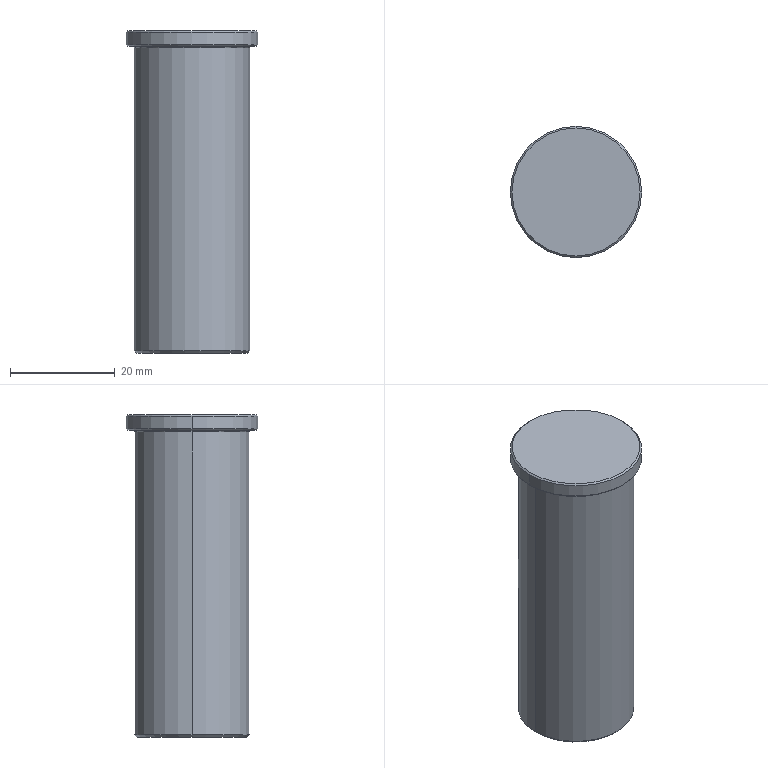Part | STEP file | Rotor step probe-10P30 | 1 solid | 20 faces | box 25 x 25 x 61.5 mm | volume 22119 mm3 | cone 8 | cylinder 6 | plane 4 | spline 2 | commonest cylinder face diameters 10 x2 22 x2 25 x2